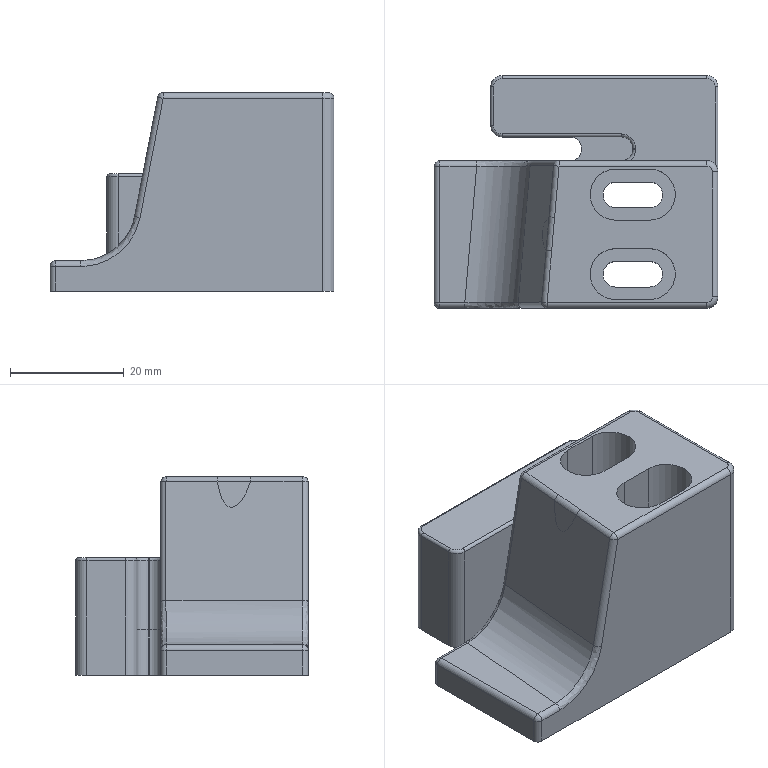Part | 1 solid | 75 faces | box 50 x 41 x 35 mm | volume 36975 mm3 | cylinder 36 | plane 26 | torus 7 | sphere 4 | spline 2 | commonest cylinder face diameters 2 x13 4 x9 1 x5 4.5 x4 9 x4 19.2 x1